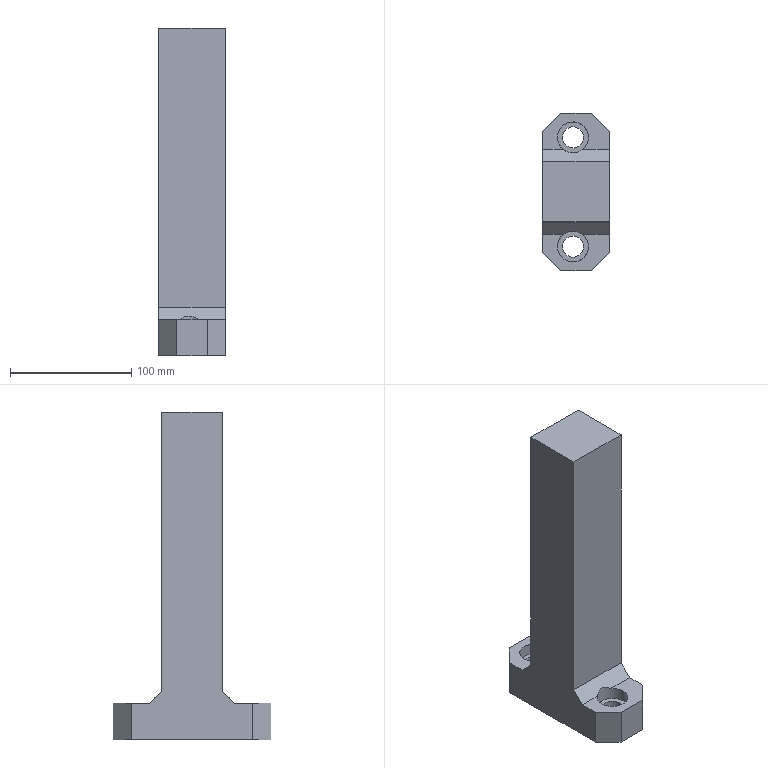Part | NX | features solid 2 | 1 solid | 22 faces | box 55 x 130 x 270 mm | volume 846599 mm3 | plane 18 | cylinder 4 | commonest cylinder face diameters 17.5 x2 25.5 x2
STEP:
#1=CARTESIAN_POINT('',(-805.,-700.,-350.));
#2=VERTEX_POINT('',#1);
#3=CARTESIAN_POINT('',(-805.,-700.,-120.));
#4=VERTEX_POINT('',#3);
#5=CARTESIAN_POINT('',(-805.,-700.,-410.));
#6=DIRECTION('',(0.,0.,1.));
#7=VECTOR('',#6,1000.);
#8=LINE('',#5,#7);
#9=EDGE_CURVE('',#2,#4,#8,.T.);
#10=ORIENTED_EDGE('',*,*,#9,.T.);
#11=CARTESIAN_POINT('',(-860.,-700.,-120.));
#12=VERTEX_POINT('',#11);
#13=CARTESIAN_POINT('',(-865.,-700.,-120.));
#14=DIRECTION('',(-1.,0.,0.));
#15=VECTOR('',#14,1000.);
#16=LINE('',#13,#15);
#17=EDGE_CURVE('',#12,#4,#16,.F.);
#18=ORIENTED_EDGE('',*,*,#17,.F.);
#19=CARTESIAN_POINT('',(-860.,-700.,-350.));
#20=VERTEX_POINT('',#19);
#21=CARTESIAN_POINT('',(-860.,-700.,-410.));
#22=DIRECTION('',(0.,0.,1.));
#23=VECTOR('',#22,1000.);
#24=LINE('',#21,#23);
#25=EDGE_CURVE('',#20,#12,#24,.T.);
#26=ORIENTED_EDGE('',*,*,#25,.F.);
#27=CARTESIAN_POINT('',(-865.,-700.,-350.));
#28=DIRECTION('',(-1.,0.,0.));
#29=VECTOR('',#28,1000.);
#30=LINE('',#27,#29);
#31=EDGE_CURVE('',#2,#20,#30,.T.);
#32=ORIENTED_EDGE('',*,*,#31,.F.);
#33=EDGE_LOOP('',(#10,#18,#26,#32));
#34=FACE_BOUND('',#33,.T.);
#35=CARTESIAN_POINT('',(-865.,-700.,-410.));
#36=DIRECTION('',(0.,1.,0.));
#37=DIRECTION('',(0.,0.,-1.));
#38=AXIS2_PLACEMENT_3D('',#35,#36,#37);
#39=PLANE('',#38);
#40=ADVANCED_FACE('',(#34),#39,.F.);
#41=CARTESIAN_POINT('',(-826.25,-720.,-390.));
#42=VERTEX_POINT('',#41);
#43=CARTESIAN_POINT('',(-835.,-720.,-390.));
#44=DIRECTION('',(0.,0.,-1.));
#45=DIRECTION('',(1.,0.,0.));
#46=AXIS2_PLACEMENT_3D('',#43,#44,#45);
#47=CIRCLE('',#46,8.75);
#48=EDGE_CURVE('',#42,#42,#47,.T.);
#49=ORIENTED_EDGE('',*,*,#48,.F.);
#50=EDGE_LOOP('',(#49));
#51=FACE_BOUND('',#50,.T.);
#52=CARTESIAN_POINT('',(-826.25,-630.,-390.));
#53=VERTEX_POINT('',#52);
#54=CARTESIAN_POINT('',(-835.,-630.,-390.));
#55=DIRECTION('',(0.,0.,-1.));
#56=DIRECTION('',(1.,0.,0.));
#57=AXIS2_PLACEMENT_3D('',#54,#55,#56);
#58=CIRCLE('',#57,8.75);
#59=EDGE_CURVE('',#53,#53,#58,.T.);
#60=ORIENTED_EDGE('',*,*,#59,.F.);
#61=EDGE_LOOP('',(#60));
#62=FACE_BOUND('',#61,.T.);
#63=CARTESIAN_POINT('',(-845.,-740.,-390.));
#64=VERTEX_POINT('',#63);
#65=CARTESIAN_POINT('',(-820.,-740.,-390.));
#66=VERTEX_POINT('',#65);
#67=CARTESIAN_POINT('',(-865.,-740.,-390.));
#68=DIRECTION('',(-1.,0.,0.));
#69=VECTOR('',#68,1000.);
#70=LINE('',#67,#69);
#71=EDGE_CURVE('',#64,#66,#70,.F.);
#72=ORIENTED_EDGE('',*,*,#71,.F.);
#73=CARTESIAN_POINT('',(-860.,-725.,-390.));
#74=VERTEX_POINT('',#73);
#75=CARTESIAN_POINT('',(-845.,-740.,-390.));
#76=DIRECTION('',(-0.7071,0.7071,0.));
#77=VECTOR('',#76,1000.);
#78=LINE('',#75,#77);
#79=EDGE_CURVE('',#74,#64,#78,.F.);
#80=ORIENTED_EDGE('',*,*,#79,.F.);
#81=CARTESIAN_POINT('',(-860.,-625.,-390.));
#82=VERTEX_POINT('',#81);
#83=CARTESIAN_POINT('',(-860.,-640.,-390.));
#84=DIRECTION('',(0.,1.,0.));
#85=VECTOR('',#84,1000.);
#86=LINE('',#83,#85);
#87=EDGE_CURVE('',#74,#82,#86,.T.);
#88=ORIENTED_EDGE('',*,*,#87,.T.);
#89=CARTESIAN_POINT('',(-845.,-610.,-390.));
#90=VERTEX_POINT('',#89);
#91=CARTESIAN_POINT('',(-860.,-625.,-390.));
#92=DIRECTION('',(-0.7071,-0.7071,0.));
#93=VECTOR('',#92,1000.);
#94=LINE('',#91,#93);
#95=EDGE_CURVE('',#90,#82,#94,.T.);
#96=ORIENTED_EDGE('',*,*,#95,.F.);
#97=CARTESIAN_POINT('',(-820.,-610.,-390.));
#98=VERTEX_POINT('',#97);
#99=CARTESIAN_POINT('',(-840.25,-610.,-390.));
#100=DIRECTION('',(1.,0.,0.));
#101=VECTOR('',#100,1000.);
#102=LINE('',#99,#101);
#103=EDGE_CURVE('',#90,#98,#102,.T.);
#104=ORIENTED_EDGE('',*,*,#103,.T.);
#105=CARTESIAN_POINT('',(-805.,-625.,-390.));
#106=VERTEX_POINT('',#105);
#107=CARTESIAN_POINT('',(-820.,-610.,-390.));
#108=DIRECTION('',(-0.7071,0.7071,0.));
#109=VECTOR('',#108,1000.);
#110=LINE('',#107,#109);
#111=EDGE_CURVE('',#106,#98,#110,.T.);
#112=ORIENTED_EDGE('',*,*,#111,.F.);
#113=CARTESIAN_POINT('',(-805.,-725.,-390.));
#114=VERTEX_POINT('',#113);
#115=CARTESIAN_POINT('',(-805.,-700.,-390.));
#116=DIRECTION('',(0.,-1.,0.));
#117=VECTOR('',#116,1000.);
#118=LINE('',#115,#117);
#119=EDGE_CURVE('',#106,#114,#118,.T.);
#120=ORIENTED_EDGE('',*,*,#119,.T.);
#121=CARTESIAN_POINT('',(-805.,-725.,-390.));
#122=DIRECTION('',(-0.7071,-0.7071,0.));
#123=VECTOR('',#122,1000.);
#124=LINE('',#121,#123);
#125=EDGE_CURVE('',#66,#114,#124,.F.);
#126=ORIENTED_EDGE('',*,*,#125,.F.);
#127=EDGE_LOOP('',(#72,#80,#88,#96,#104,#112,#120,#126));
#128=FACE_BOUND('',#127,.T.);
#129=CARTESIAN_POINT('',(-840.25,-840.,-390.));
#130=DIRECTION('',(0.,0.,1.));
#131=DIRECTION('',(1.,0.,0.));
#132=AXIS2_PLACEMENT_3D('',#129,#130,#131);
#133=PLANE('',#132);
#134=ADVANCED_FACE('',(#51,#62,#128),#133,.F.);
#135=CARTESIAN_POINT('',(-860.,-650.,-350.));
#136=VERTEX_POINT('',#135);
#137=CARTESIAN_POINT('',(-860.,-650.,-120.));
#138=VERTEX_POINT('',#137);
#139=CARTESIAN_POINT('',(-860.,-650.,-410.));
#140=DIRECTION('',(0.,0.,1.));
#141=VECTOR('',#140,1000.);
#142=LINE('',#139,#141);
#143=EDGE_CURVE('',#136,#138,#142,.T.);
#144=ORIENTED_EDGE('',*,*,#143,.T.);
#145=CARTESIAN_POINT('',(-805.,-650.,-120.));
#146=VERTEX_POINT('',#145);
#147=CARTESIAN_POINT('',(-800.,-650.,-120.));
#148=DIRECTION('',(1.,0.,0.));
#149=VECTOR('',#148,1000.);
#150=LINE('',#147,#149);
#151=EDGE_CURVE('',#146,#138,#150,.F.);
#152=ORIENTED_EDGE('',*,*,#151,.F.);
#153=CARTESIAN_POINT('',(-805.,-650.,-350.));
#154=VERTEX_POINT('',#153);
#155=CARTESIAN_POINT('',(-805.,-650.,-410.));
#156=DIRECTION('',(0.,0.,1.));
#157=VECTOR('',#156,1000.);
#158=LINE('',#155,#157);
#159=EDGE_CURVE('',#154,#146,#158,.T.);
#160=ORIENTED_EDGE('',*,*,#159,.F.);
#161=CARTESIAN_POINT('',(-800.,-650.,-350.));
#162=DIRECTION('',(1.,0.,0.));
#163=VECTOR('',#162,1000.);
#164=LINE('',#161,#163);
#165=EDGE_CURVE('',#136,#154,#164,.T.);
#166=ORIENTED_EDGE('',*,*,#165,.F.);
#167=EDGE_LOOP('',(#144,#152,#160,#166));
#168=FACE_BOUND('',#167,.T.);
#169=CARTESIAN_POINT('',(-800.,-650.,-410.));
#170=DIRECTION('',(0.,-1.,0.));
#171=DIRECTION('',(0.,0.,1.));
#172=AXIS2_PLACEMENT_3D('',#169,#170,#171);
#173=PLANE('',#172);
#174=ADVANCED_FACE('',(#168),#173,.F.);
#175=ORIENTED_EDGE('',*,*,#87,.F.);
#176=CARTESIAN_POINT('',(-860.,-725.,-360.));
#177=VERTEX_POINT('',#176);
#178=CARTESIAN_POINT('',(-860.,-725.,-390.));
#179=DIRECTION('',(0.,0.,-1.));
#180=VECTOR('',#179,1000.);
#181=LINE('',#178,#180);
#182=EDGE_CURVE('',#177,#74,#181,.T.);
#183=ORIENTED_EDGE('',*,*,#182,.F.);
#184=CARTESIAN_POINT('',(-860.,-710.,-360.));
#185=VERTEX_POINT('',#184);
#186=CARTESIAN_POINT('',(-860.,-705.,-360.));
#187=DIRECTION('',(0.,-1.,0.));
#188=VECTOR('',#187,1000.);
#189=LINE('',#186,#188);
#190=EDGE_CURVE('',#185,#177,#189,.T.);
#191=ORIENTED_EDGE('',*,*,#190,.F.);
#192=CARTESIAN_POINT('',(-860.,-700.,-350.));
#193=DIRECTION('',(0.,-0.7071,-0.7071));
#194=VECTOR('',#193,1000.);
#195=LINE('',#192,#194);
#196=EDGE_CURVE('',#20,#185,#195,.T.);
#197=ORIENTED_EDGE('',*,*,#196,.F.);
#198=ORIENTED_EDGE('',*,*,#25,.T.);
#199=CARTESIAN_POINT('',(-860.,-640.,-120.));
#200=DIRECTION('',(0.,1.,0.));
#201=VECTOR('',#200,1000.);
#202=LINE('',#199,#201);
#203=EDGE_CURVE('',#138,#12,#202,.F.);
#204=ORIENTED_EDGE('',*,*,#203,.F.);
#205=ORIENTED_EDGE('',*,*,#143,.F.);
#206=CARTESIAN_POINT('',(-860.,-640.,-360.));
#207=VERTEX_POINT('',#206);
#208=CARTESIAN_POINT('',(-860.,-615.,-385.));
#209=DIRECTION('',(0.,-0.7071,0.7071));
#210=VECTOR('',#209,1000.);
#211=LINE('',#208,#210);
#212=EDGE_CURVE('',#207,#136,#211,.T.);
#213=ORIENTED_EDGE('',*,*,#212,.F.);
#214=CARTESIAN_POINT('',(-860.,-625.,-360.));
#215=VERTEX_POINT('',#214);
#216=CARTESIAN_POINT('',(-860.,-610.,-360.));
#217=DIRECTION('',(0.,-1.,0.));
#218=VECTOR('',#217,1000.);
#219=LINE('',#216,#218);
#220=EDGE_CURVE('',#215,#207,#219,.T.);
#221=ORIENTED_EDGE('',*,*,#220,.F.);
#222=CARTESIAN_POINT('',(-860.,-625.,-360.));
#223=DIRECTION('',(0.,0.,1.));
#224=VECTOR('',#223,1000.);
#225=LINE('',#222,#224);
#226=EDGE_CURVE('',#82,#215,#225,.T.);
#227=ORIENTED_EDGE('',*,*,#226,.F.);
#228=EDGE_LOOP('',(#175,#183,#191,#197,#198,#204,#205,#213,#221,#227));
#229=FACE_BOUND('',#228,.T.);
#230=CARTESIAN_POINT('',(-860.,-640.,-410.));
#231=DIRECTION('',(1.,0.,0.));
#232=DIRECTION('',(0.,0.,-1.));
#233=AXIS2_PLACEMENT_3D('',#230,#231,#232);
#234=PLANE('',#233);
#235=ADVANCED_FACE('',(#229),#234,.F.);
#236=ORIENTED_EDGE('',*,*,#119,.F.);
#237=CARTESIAN_POINT('',(-805.,-625.,-360.));
#238=VERTEX_POINT('',#237);
#239=CARTESIAN_POINT('',(-805.,-625.,-390.));
#240=DIRECTION('',(0.,0.,-1.));
#241=VECTOR('',#240,1000.);
#242=LINE('',#239,#241);
#243=EDGE_CURVE('',#238,#106,#242,.T.);
#244=ORIENTED_EDGE('',*,*,#243,.F.);
#245=CARTESIAN_POINT('',(-805.,-640.,-360.));
#246=VERTEX_POINT('',#245);
#247=CARTESIAN_POINT('',(-805.,-700.,-360.));
#248=DIRECTION('',(0.,-1.,0.));
#249=VECTOR('',#248,1000.);
#250=LINE('',#247,#249);
#251=EDGE_CURVE('',#238,#246,#250,.T.);
#252=ORIENTED_EDGE('',*,*,#251,.T.);
#253=CARTESIAN_POINT('',(-805.,-645.,-355.));
#254=DIRECTION('',(0.,0.7071,-0.7071));
#255=VECTOR('',#254,1000.);
#256=LINE('',#253,#255);
#257=EDGE_CURVE('',#154,#246,#256,.T.);
#258=ORIENTED_EDGE('',*,*,#257,.F.);
#259=ORIENTED_EDGE('',*,*,#159,.T.);
#260=CARTESIAN_POINT('',(-805.,-700.,-120.));
#261=DIRECTION('',(0.,-1.,0.));
#262=VECTOR('',#261,1000.);
#263=LINE('',#260,#262);
#264=EDGE_CURVE('',#4,#146,#263,.F.);
#265=ORIENTED_EDGE('',*,*,#264,.F.);
#266=ORIENTED_EDGE('',*,*,#9,.F.);
#267=CARTESIAN_POINT('',(-805.,-710.,-360.));
#268=VERTEX_POINT('',#267);
#269=CARTESIAN_POINT('',(-805.,-730.,-380.));
#270=DIRECTION('',(0.,0.7071,0.7071));
#271=VECTOR('',#270,1000.);
#272=LINE('',#269,#271);
#273=EDGE_CURVE('',#268,#2,#272,.T.);
#274=ORIENTED_EDGE('',*,*,#273,.F.);
#275=CARTESIAN_POINT('',(-805.,-725.,-360.));
#276=VERTEX_POINT('',#275);
#277=CARTESIAN_POINT('',(-805.,-705.,-360.));
#278=DIRECTION('',(0.,-1.,0.));
#279=VECTOR('',#278,1000.);
#280=LINE('',#277,#279);
#281=EDGE_CURVE('',#268,#276,#280,.T.);
#282=ORIENTED_EDGE('',*,*,#281,.T.);
#283=CARTESIAN_POINT('',(-805.,-725.,-360.));
#284=DIRECTION('',(0.,0.,1.));
#285=VECTOR('',#284,1000.);
#286=LINE('',#283,#285);
#287=EDGE_CURVE('',#114,#276,#286,.T.);
#288=ORIENTED_EDGE('',*,*,#287,.F.);
#289=EDGE_LOOP('',(#236,#244,#252,#258,#259,#265,#266,#274,#282,#288));
#290=FACE_BOUND('',#289,.T.);
#291=CARTESIAN_POINT('',(-805.,-700.,-410.));
#292=DIRECTION('',(-1.,0.,0.));
#293=DIRECTION('',(0.,0.,1.));
#294=AXIS2_PLACEMENT_3D('',#291,#292,#293);
#295=PLANE('',#294);
#296=ADVANCED_FACE('',(#290),#295,.F.);
#297=ORIENTED_EDGE('',*,*,#151,.T.);
#298=ORIENTED_EDGE('',*,*,#203,.T.);
#299=ORIENTED_EDGE('',*,*,#17,.T.);
#300=ORIENTED_EDGE('',*,*,#264,.T.);
#301=EDGE_LOOP('',(#297,#298,#299,#300));
#302=FACE_BOUND('',#301,.T.);
#303=CARTESIAN_POINT('',(0.,20.049,-120.));
#304=DIRECTION('',(0.,0.,1.));
#305=DIRECTION('',(-1.,0.,0.));
#306=AXIS2_PLACEMENT_3D('',#303,#304,#305);
#307=PLANE('',#306);
#308=ADVANCED_FACE('',(#302),#307,.T.);
#309=CARTESIAN_POINT('',(-845.,-740.,-360.));
#310=VERTEX_POINT('',#309);
#311=CARTESIAN_POINT('',(-820.,-740.,-360.));
#312=VERTEX_POINT('',#311);
#313=CARTESIAN_POINT('',(-865.,-740.,-360.));
#314=DIRECTION('',(-1.,0.,0.));
#315=VECTOR('',#314,1000.);
#316=LINE('',#313,#315);
#317=EDGE_CURVE('',#310,#312,#316,.F.);
#318=ORIENTED_EDGE('',*,*,#317,.F.);
#319=CARTESIAN_POINT('',(-845.,-740.,-360.));
#320=DIRECTION('',(0.,0.,-1.));
#321=VECTOR('',#320,1000.);
#322=LINE('',#319,#321);
#323=EDGE_CURVE('',#64,#310,#322,.F.);
#324=ORIENTED_EDGE('',*,*,#323,.F.);
#325=ORIENTED_EDGE('',*,*,#71,.T.);
#326=CARTESIAN_POINT('',(-820.,-740.,-390.));
#327=DIRECTION('',(0.,0.,1.));
#328=VECTOR('',#327,1000.);
#329=LINE('',#326,#328);
#330=EDGE_CURVE('',#312,#66,#329,.F.);
#331=ORIENTED_EDGE('',*,*,#330,.F.);
#332=EDGE_LOOP('',(#318,#324,#325,#331));
#333=FACE_BOUND('',#332,.T.);
#334=CARTESIAN_POINT('',(-865.,-740.,-380.));
#335=DIRECTION('',(0.,1.,0.));
#336=DIRECTION('',(1.,0.,0.));
#337=AXIS2_PLACEMENT_3D('',#334,#335,#336);
#338=PLANE('',#337);
#339=ADVANCED_FACE('',(#333),#338,.F.);
#340=ORIENTED_EDGE('',*,*,#190,.T.);
#341=CARTESIAN_POINT('',(-870.,-715.,-360.));
#342=DIRECTION('',(0.7071,-0.7071,0.));
#343=VECTOR('',#342,1000.);
#344=LINE('',#341,#343);
#345=EDGE_CURVE('',#310,#177,#344,.F.);
#346=ORIENTED_EDGE('',*,*,#345,.F.);
#347=ORIENTED_EDGE('',*,*,#317,.T.);
#348=CARTESIAN_POINT('',(-827.5,-747.5,-360.));
#349=DIRECTION('',(0.7071,0.7071,0.));
#350=VECTOR('',#349,1000.);
#351=LINE('',#348,#350);
#352=EDGE_CURVE('',#276,#312,#351,.F.);
#353=ORIENTED_EDGE('',*,*,#352,.F.);
#354=ORIENTED_EDGE('',*,*,#281,.F.);
#355=CARTESIAN_POINT('',(-827.09,-710.,-360.));
#356=VERTEX_POINT('',#355);
#357=CARTESIAN_POINT('',(-865.,-710.,-360.));
#358=DIRECTION('',(1.,0.,0.));
#359=VECTOR('',#358,1000.);
#360=LINE('',#357,#359);
#361=EDGE_CURVE('',#356,#268,#360,.T.);
#362=ORIENTED_EDGE('',*,*,#361,.F.);
#363=CARTESIAN_POINT('',(-842.91,-710.,-360.));
#364=VERTEX_POINT('',#363);
#365=CARTESIAN_POINT('',(-835.,-720.,-360.));
#366=DIRECTION('',(0.,0.,1.));
#367=DIRECTION('',(-1.,0.,0.));
#368=AXIS2_PLACEMENT_3D('',#365,#366,#367);
#369=CIRCLE('',#368,12.75);
#370=EDGE_CURVE('',#364,#356,#369,.T.);
#371=ORIENTED_EDGE('',*,*,#370,.F.);
#372=CARTESIAN_POINT('',(-865.,-710.,-360.));
#373=DIRECTION('',(1.,0.,0.));
#374=VECTOR('',#373,1000.);
#375=LINE('',#372,#374);
#376=EDGE_CURVE('',#185,#364,#375,.T.);
#377=ORIENTED_EDGE('',*,*,#376,.F.);
#378=EDGE_LOOP('',(#340,#346,#347,#353,#354,#362,#371,#377));
#379=FACE_BOUND('',#378,.T.);
#380=CARTESIAN_POINT('',(-865.,-710.,-360.));
#381=DIRECTION('',(0.,0.,1.));
#382=DIRECTION('',(1.,0.,0.));
#383=AXIS2_PLACEMENT_3D('',#380,#381,#382);
#384=PLANE('',#383);
#385=ADVANCED_FACE('',(#379),#384,.T.);
#386=ORIENTED_EDGE('',*,*,#103,.F.);
#387=CARTESIAN_POINT('',(-845.,-610.,-360.));
#388=VERTEX_POINT('',#387);
#389=CARTESIAN_POINT('',(-845.,-610.,-390.));
#390=DIRECTION('',(0.,0.,-1.));
#391=VECTOR('',#390,1000.);
#392=LINE('',#389,#391);
#393=EDGE_CURVE('',#388,#90,#392,.T.);
#394=ORIENTED_EDGE('',*,*,#393,.F.);
#395=CARTESIAN_POINT('',(-820.,-610.,-360.));
#396=VERTEX_POINT('',#395);
#397=CARTESIAN_POINT('',(-865.,-610.,-360.));
#398=DIRECTION('',(1.,0.,0.));
#399=VECTOR('',#398,1000.);
#400=LINE('',#397,#399);
#401=EDGE_CURVE('',#388,#396,#400,.T.);
#402=ORIENTED_EDGE('',*,*,#401,.T.);
#403=CARTESIAN_POINT('',(-820.,-610.,-360.));
#404=DIRECTION('',(0.,0.,1.));
#405=VECTOR('',#404,1000.);
#406=LINE('',#403,#405);
#407=EDGE_CURVE('',#98,#396,#406,.T.);
#408=ORIENTED_EDGE('',*,*,#407,.F.);
#409=EDGE_LOOP('',(#386,#394,#402,#408));
#410=FACE_BOUND('',#409,.T.);
#411=CARTESIAN_POINT('',(-865.,-610.,-380.));
#412=DIRECTION('',(0.,1.,0.));
#413=DIRECTION('',(1.,0.,0.));
#414=AXIS2_PLACEMENT_3D('',#411,#412,#413);
#415=PLANE('',#414);
#416=ADVANCED_FACE('',(#410),#415,.T.);
#417=ORIENTED_EDGE('',*,*,#251,.F.);
#418=CARTESIAN_POINT('',(-842.5,-587.5,-360.));
#419=DIRECTION('',(0.7071,-0.7071,0.));
#420=VECTOR('',#419,1000.);
#421=LINE('',#418,#420);
#422=EDGE_CURVE('',#396,#238,#421,.T.);
#423=ORIENTED_EDGE('',*,*,#422,.F.);
#424=ORIENTED_EDGE('',*,*,#401,.F.);
#425=CARTESIAN_POINT('',(-855.,-620.,-360.));
#426=DIRECTION('',(0.7071,0.7071,0.));
#427=VECTOR('',#426,1000.);
#428=LINE('',#425,#427);
#429=EDGE_CURVE('',#215,#388,#428,.T.);
#430=ORIENTED_EDGE('',*,*,#429,.F.);
#431=ORIENTED_EDGE('',*,*,#220,.T.);
#432=CARTESIAN_POINT('',(-842.91,-640.,-360.));
#433=VERTEX_POINT('',#432);
#434=CARTESIAN_POINT('',(-865.,-640.,-360.));
#435=DIRECTION('',(-1.,0.,0.));
#436=VECTOR('',#435,1000.);
#437=LINE('',#434,#436);
#438=EDGE_CURVE('',#433,#207,#437,.T.);
#439=ORIENTED_EDGE('',*,*,#438,.F.);
#440=CARTESIAN_POINT('',(-827.09,-640.,-360.));
#441=VERTEX_POINT('',#440);
#442=CARTESIAN_POINT('',(-835.,-630.,-360.));
#443=DIRECTION('',(0.,0.,1.));
#444=DIRECTION('',(-1.,0.,0.));
#445=AXIS2_PLACEMENT_3D('',#442,#443,#444);
#446=CIRCLE('',#445,12.75);
#447=EDGE_CURVE('',#441,#433,#446,.T.);
#448=ORIENTED_EDGE('',*,*,#447,.F.);
#449=CARTESIAN_POINT('',(-865.,-640.,-360.));
#450=DIRECTION('',(-1.,0.,0.));
#451=VECTOR('',#450,1000.);
#452=LINE('',#449,#451);
#453=EDGE_CURVE('',#246,#441,#452,.T.);
#454=ORIENTED_EDGE('',*,*,#453,.F.);
#455=EDGE_LOOP('',(#417,#423,#424,#430,#431,#439,#448,#454));
#456=FACE_BOUND('',#455,.T.);
#457=CARTESIAN_POINT('',(-865.,-610.,-360.));
#458=DIRECTION('',(0.,0.,1.));
#459=DIRECTION('',(1.,0.,0.));
#460=AXIS2_PLACEMENT_3D('',#457,#458,#459);
#461=PLANE('',#460);
#462=ADVANCED_FACE('',(#456),#461,.T.);
#463=CARTESIAN_POINT('',(-843.75,-630.,-370.));
#464=VERTEX_POINT('',#463);
#465=CARTESIAN_POINT('',(-835.,-630.,-370.));
#466=DIRECTION('',(0.,0.,1.));
#467=DIRECTION('',(-1.,0.,0.));
#468=AXIS2_PLACEMENT_3D('',#465,#466,#467);
#469=CIRCLE('',#468,8.75);
#470=EDGE_CURVE('',#464,#464,#469,.T.);
#471=ORIENTED_EDGE('',*,*,#470,.T.);
#472=EDGE_LOOP('',(#471));
#473=FACE_BOUND('',#472,.T.);
#474=ORIENTED_EDGE('',*,*,#59,.T.);
#475=EDGE_LOOP('',(#474));
#476=FACE_BOUND('',#475,.T.);
#477=CARTESIAN_POINT('',(-835.,-630.,-410.));
#478=DIRECTION('',(0.,0.,-1.));
#479=DIRECTION('',(-1.,0.,0.));
#480=AXIS2_PLACEMENT_3D('',#477,#478,#479);
#481=CYLINDRICAL_SURFACE('',#480,8.75);
#482=ADVANCED_FACE('',(#473,#476),#481,.F.);
#483=ORIENTED_EDGE('',*,*,#470,.F.);
#484=EDGE_LOOP('',(#483));
#485=FACE_BOUND('',#484,.T.);
#486=CARTESIAN_POINT('',(-847.75,-630.,-370.));
#487=VERTEX_POINT('',#486);
#488=CARTESIAN_POINT('',(-835.,-630.,-370.));
#489=DIRECTION('',(0.,0.,1.));
#490=DIRECTION('',(-1.,0.,0.));
#491=AXIS2_PLACEMENT_3D('',#488,#489,#490);
#492=CIRCLE('',#491,12.75);
#493=EDGE_CURVE('',#487,#487,#492,.T.);
#494=ORIENTED_EDGE('',*,*,#493,.T.);
#495=EDGE_LOOP('',(#494));
#496=FACE_BOUND('',#495,.T.);
#497=CARTESIAN_POINT('',(-835.,-630.,-370.));
#498=DIRECTION('',(0.,0.,-1.));
#499=DIRECTION('',(-1.,0.,0.));
#500=AXIS2_PLACEMENT_3D('',#497,#498,#499);
#501=PLANE('',#500);
#502=ADVANCED_FACE('',(#485,#496),#501,.F.);
#503=ORIENTED_EDGE('',*,*,#493,.F.);
#504=EDGE_LOOP('',(#503));
#505=FACE_BOUND('',#504,.T.);
#506=ORIENTED_EDGE('',*,*,#447,.T.);
#507=CARTESIAN_POINT('',(-835.,-630.,-370.));
#508=DIRECTION('',(0.,0.7071,0.7071));
#509=DIRECTION('',(0.,0.7071,-0.7071));
#510=AXIS2_PLACEMENT_3D('',#507,#508,#509);
#511=ELLIPSE('',#510,18.031,12.75);
#512=EDGE_CURVE('',#441,#433,#511,.F.);
#513=ORIENTED_EDGE('',*,*,#512,.F.);
#514=EDGE_LOOP('',(#506,#513));
#515=FACE_BOUND('',#514,.T.);
#516=CARTESIAN_POINT('',(-835.,-630.,-360.));
#517=DIRECTION('',(0.,0.,-1.));
#518=DIRECTION('',(-1.,0.,0.));
#519=AXIS2_PLACEMENT_3D('',#516,#517,#518);
#520=CYLINDRICAL_SURFACE('',#519,12.75);
#521=ADVANCED_FACE('',(#505,#515),#520,.F.);
#522=CARTESIAN_POINT('',(-843.75,-720.,-370.));
#523=VERTEX_POINT('',#522);
#524=CARTESIAN_POINT('',(-835.,-720.,-370.));
#525=DIRECTION('',(0.,0.,1.));
#526=DIRECTION('',(-1.,0.,0.));
#527=AXIS2_PLACEMENT_3D('',#524,#525,#526);
#528=CIRCLE('',#527,8.75);
#529=EDGE_CURVE('',#523,#523,#528,.T.);
#530=ORIENTED_EDGE('',*,*,#529,.T.);
#531=EDGE_LOOP('',(#530));
#532=FACE_BOUND('',#531,.T.);
#533=ORIENTED_EDGE('',*,*,#48,.T.);
#534=EDGE_LOOP('',(#533));
#535=FACE_BOUND('',#534,.T.);
#536=CARTESIAN_POINT('',(-835.,-720.,-410.));
#537=DIRECTION('',(0.,0.,-1.));
#538=DIRECTION('',(-1.,0.,0.));
#539=AXIS2_PLACEMENT_3D('',#536,#537,#538);
#540=CYLINDRICAL_SURFACE('',#539,8.75);
#541=ADVANCED_FACE('',(#532,#535),#540,.F.);
#542=ORIENTED_EDGE('',*,*,#529,.F.);
#543=EDGE_LOOP('',(#542));
#544=FACE_BOUND('',#543,.T.);
#545=CARTESIAN_POINT('',(-847.75,-720.,-370.));
#546=VERTEX_POINT('',#545);
#547=CARTESIAN_POINT('',(-835.,-720.,-370.));
#548=DIRECTION('',(0.,0.,1.));
#549=DIRECTION('',(-1.,0.,0.));
#550=AXIS2_PLACEMENT_3D('',#547,#548,#549);
#551=CIRCLE('',#550,12.75);
#552=EDGE_CURVE('',#546,#546,#551,.T.);
#553=ORIENTED_EDGE('',*,*,#552,.T.);
#554=EDGE_LOOP('',(#553));
#555=FACE_BOUND('',#554,.T.);
#556=CARTESIAN_POINT('',(-835.,-720.,-370.));
#557=DIRECTION('',(0.,0.,-1.));
#558=DIRECTION('',(-1.,0.,0.));
#559=AXIS2_PLACEMENT_3D('',#556,#557,#558);
#560=PLANE('',#559);
#561=ADVANCED_FACE('',(#544,#555),#560,.F.);
#562=ORIENTED_EDGE('',*,*,#552,.F.);
#563=EDGE_LOOP('',(#562));
#564=FACE_BOUND('',#563,.T.);
#565=ORIENTED_EDGE('',*,*,#370,.T.);
#566=CARTESIAN_POINT('',(-835.,-720.,-370.));
#567=DIRECTION('',(0.,-0.7071,0.7071));
#568=DIRECTION('',(0.,-0.7071,-0.7071));
#569=AXIS2_PLACEMENT_3D('',#566,#567,#568);
#570=ELLIPSE('',#569,18.031,12.75);
#571=EDGE_CURVE('',#364,#356,#570,.F.);
#572=ORIENTED_EDGE('',*,*,#571,.F.);
#573=EDGE_LOOP('',(#565,#572));
#574=FACE_BOUND('',#573,.T.);
#575=CARTESIAN_POINT('',(-835.,-720.,-360.));
#576=DIRECTION('',(0.,0.,-1.));
#577=DIRECTION('',(-1.,0.,0.));
#578=AXIS2_PLACEMENT_3D('',#575,#576,#577);
#579=CYLINDRICAL_SURFACE('',#578,12.75);
#580=ADVANCED_FACE('',(#564,#574),#579,.F.);
#581=ORIENTED_EDGE('',*,*,#79,.T.);
#582=ORIENTED_EDGE('',*,*,#323,.T.);
#583=ORIENTED_EDGE('',*,*,#345,.T.);
#584=ORIENTED_EDGE('',*,*,#182,.T.);
#585=EDGE_LOOP('',(#581,#582,#583,#584));
#586=FACE_BOUND('',#585,.T.);
#587=CARTESIAN_POINT('',(-845.,-740.,-380.));
#588=DIRECTION('',(0.7071,0.7071,0.));
#589=DIRECTION('',(0.7071,-0.7071,0.));
#590=AXIS2_PLACEMENT_3D('',#587,#588,#589);
#591=PLANE('',#590);
#592=ADVANCED_FACE('',(#586),#591,.F.);
#593=ORIENTED_EDGE('',*,*,#95,.T.);
#594=ORIENTED_EDGE('',*,*,#226,.T.);
#595=ORIENTED_EDGE('',*,*,#429,.T.);
#596=ORIENTED_EDGE('',*,*,#393,.T.);
#597=EDGE_LOOP('',(#593,#594,#595,#596));
#598=FACE_BOUND('',#597,.T.);
#599=CARTESIAN_POINT('',(-860.,-625.,-410.));
#600=DIRECTION('',(-0.7071,0.7071,0.));
#601=DIRECTION('',(0.7071,0.7071,0.));
#602=AXIS2_PLACEMENT_3D('',#599,#600,#601);
#603=PLANE('',#602);
#604=ADVANCED_FACE('',(#598),#603,.T.);
#605=ORIENTED_EDGE('',*,*,#125,.T.);
#606=ORIENTED_EDGE('',*,*,#287,.T.);
#607=ORIENTED_EDGE('',*,*,#352,.T.);
#608=ORIENTED_EDGE('',*,*,#330,.T.);
#609=EDGE_LOOP('',(#605,#606,#607,#608));
#610=FACE_BOUND('',#609,.T.);
#611=CARTESIAN_POINT('',(-805.,-725.,-410.));
#612=DIRECTION('',(-0.7071,0.7071,0.));
#613=DIRECTION('',(0.7071,0.7071,0.));
#614=AXIS2_PLACEMENT_3D('',#611,#612,#613);
#615=PLANE('',#614);
#616=ADVANCED_FACE('',(#610),#615,.F.);
#617=ORIENTED_EDGE('',*,*,#111,.T.);
#618=ORIENTED_EDGE('',*,*,#407,.T.);
#619=ORIENTED_EDGE('',*,*,#422,.T.);
#620=ORIENTED_EDGE('',*,*,#243,.T.);
#621=EDGE_LOOP('',(#617,#618,#619,#620));
#622=FACE_BOUND('',#621,.T.);
#623=CARTESIAN_POINT('',(-820.,-610.,-380.));
#624=DIRECTION('',(0.7071,0.7071,0.));
#625=DIRECTION('',(0.7071,-0.7071,0.));
#626=AXIS2_PLACEMENT_3D('',#623,#624,#625);
#627=PLANE('',#626);
#628=ADVANCED_FACE('',(#622),#627,.T.);
#629=ORIENTED_EDGE('',*,*,#196,.T.);
#630=ORIENTED_EDGE('',*,*,#376,.T.);
#631=ORIENTED_EDGE('',*,*,#571,.T.);
#632=ORIENTED_EDGE('',*,*,#361,.T.);
#633=ORIENTED_EDGE('',*,*,#273,.T.);
#634=ORIENTED_EDGE('',*,*,#31,.T.);
#635=EDGE_LOOP('',(#629,#630,#631,#632,#633,#634));
#636=FACE_BOUND('',#635,.T.);
#637=CARTESIAN_POINT('',(-865.,-710.,-360.));
#638=DIRECTION('',(0.,0.7071,-0.7071));
#639=DIRECTION('',(0.,-0.7071,-0.7071));
#640=AXIS2_PLACEMENT_3D('',#637,#638,#639);
#641=PLANE('',#640);
#642=ADVANCED_FACE('',(#636),#641,.F.);
#643=ORIENTED_EDGE('',*,*,#512,.T.);
#644=ORIENTED_EDGE('',*,*,#438,.T.);
#645=ORIENTED_EDGE('',*,*,#212,.T.);
#646=ORIENTED_EDGE('',*,*,#165,.T.);
#647=ORIENTED_EDGE('',*,*,#257,.T.);
#648=ORIENTED_EDGE('',*,*,#453,.T.);
#649=EDGE_LOOP('',(#643,#644,#645,#646,#647,#648));
#650=FACE_BOUND('',#649,.T.);
#651=CARTESIAN_POINT('',(-800.,-650.,-350.));
#652=DIRECTION('',(0.,-0.7071,-0.7071));
#653=DIRECTION('',(0.,-0.7071,0.7071));
#654=AXIS2_PLACEMENT_3D('',#651,#652,#653);
#655=PLANE('',#654);
#656=ADVANCED_FACE('',(#650),#655,.F.);
#657=CLOSED_SHELL('',(#40,#134,#174,#235,#296,#308,#339,#385,#416,#462,#482,#502,#521,#541,#561,#580,#592,#604,#616,#628,#642,#656));
#658=MANIFOLD_SOLID_BREP('',#657);
#659=(LENGTH_UNIT()NAMED_UNIT(*)SI_UNIT(.MILLI.,.METRE.));
#660=UNCERTAINTY_MEASURE_WITH_UNIT(LENGTH_MEASURE(0.00001),#659,'','');
#661=(NAMED_UNIT(*)PLANE_ANGLE_UNIT()SI_UNIT($,.RADIAN.));
#662=(NAMED_UNIT(*)SI_UNIT($,.STERADIAN.)SOLID_ANGLE_UNIT());
#663=(GEOMETRIC_REPRESENTATION_CONTEXT(3)GLOBAL_UNCERTAINTY_ASSIGNED_CONTEXT((#660))GLOBAL_UNIT_ASSIGNED_CONTEXT((#659,#661,#662))REPRESENTATION_CONTEXT('',''));
#664=ADVANCED_BREP_SHAPE_REPRESENTATION('',(#658),#663);